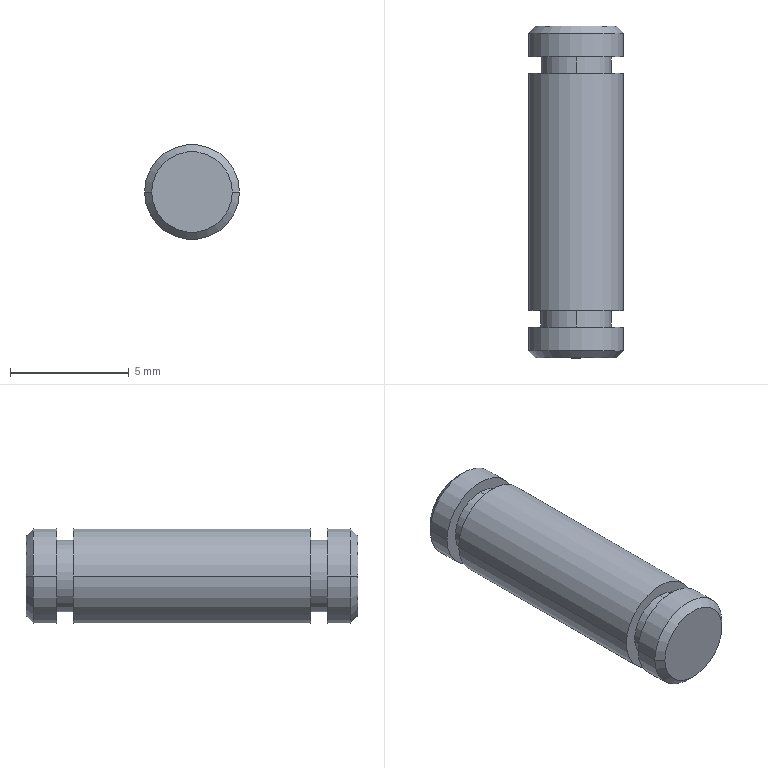Part | NX | 1 solid | 20 faces | box 4 x 14 x 4 mm | volume 167.158 mm3 | cylinder 10 | plane 6 | cone 4 | commonest cylinder face diameters 4 x6 3 x4
STEP:
#1=CARTESIAN_POINT('',(-42.,151.3,-84.4));
#2=VERTEX_POINT('',#1);
#3=CARTESIAN_POINT('',(-46.,151.3,-84.4));
#4=VERTEX_POINT('',#3);
#5=CARTESIAN_POINT('',(-44.,151.3,-84.4));
#6=DIRECTION('',(0.,1.,0.));
#7=DIRECTION('',(-1.,0.,0.));
#8=AXIS2_PLACEMENT_3D('',#5,#6,#7);
#9=CIRCLE('',#8,2.);
#10=EDGE_CURVE('',#2,#4,#9,.T.);
#11=ORIENTED_EDGE('',*,*,#10,.T.);
#12=CARTESIAN_POINT('',(-46.,152.3,-84.4));
#13=VERTEX_POINT('',#12);
#14=CARTESIAN_POINT('',(-46.,165.,-84.4));
#15=DIRECTION('',(0.,1.,0.));
#16=VECTOR('',#15,1000.);
#17=LINE('',#14,#16);
#18=EDGE_CURVE('',#4,#13,#17,.T.);
#19=ORIENTED_EDGE('',*,*,#18,.T.);
#20=CARTESIAN_POINT('',(-42.,152.3,-84.4));
#21=VERTEX_POINT('',#20);
#22=CARTESIAN_POINT('',(-44.,152.3,-84.4));
#23=DIRECTION('',(0.,1.,0.));
#24=DIRECTION('',(-1.,0.,0.));
#25=AXIS2_PLACEMENT_3D('',#22,#23,#24);
#26=CIRCLE('',#25,2.);
#27=EDGE_CURVE('',#21,#13,#26,.T.);
#28=ORIENTED_EDGE('',*,*,#27,.F.);
#29=CARTESIAN_POINT('',(-42.,165.,-84.4));
#30=DIRECTION('',(0.,1.,0.));
#31=VECTOR('',#30,1000.);
#32=LINE('',#29,#31);
#33=EDGE_CURVE('',#2,#21,#32,.T.);
#34=ORIENTED_EDGE('',*,*,#33,.F.);
#35=EDGE_LOOP('',(#11,#19,#28,#34));
#36=FACE_BOUND('',#35,.T.);
#37=CARTESIAN_POINT('',(-44.,165.,-84.4));
#38=DIRECTION('',(0.,1.,0.));
#39=DIRECTION('',(-1.,0.,0.));
#40=AXIS2_PLACEMENT_3D('',#37,#38,#39);
#41=CYLINDRICAL_SURFACE('',#40,2.);
#42=ADVANCED_FACE('',(#36),#41,.T.);
#43=CARTESIAN_POINT('',(-42.,163.7,-84.4));
#44=VERTEX_POINT('',#43);
#45=CARTESIAN_POINT('',(-46.,163.7,-84.4));
#46=VERTEX_POINT('',#45);
#47=CARTESIAN_POINT('',(-44.,163.7,-84.4));
#48=DIRECTION('',(0.,1.,0.));
#49=DIRECTION('',(-1.,0.,0.));
#50=AXIS2_PLACEMENT_3D('',#47,#48,#49);
#51=CIRCLE('',#50,2.);
#52=EDGE_CURVE('',#44,#46,#51,.T.);
#53=ORIENTED_EDGE('',*,*,#52,.T.);
#54=CARTESIAN_POINT('',(-46.,164.7,-84.4));
#55=VERTEX_POINT('',#54);
#56=CARTESIAN_POINT('',(-46.,165.,-84.4));
#57=DIRECTION('',(0.,1.,0.));
#58=VECTOR('',#57,1000.);
#59=LINE('',#56,#58);
#60=EDGE_CURVE('',#55,#46,#59,.F.);
#61=ORIENTED_EDGE('',*,*,#60,.F.);
#62=CARTESIAN_POINT('',(-42.,164.7,-84.4));
#63=VERTEX_POINT('',#62);
#64=CARTESIAN_POINT('',(-44.,164.7,-84.4));
#65=DIRECTION('',(0.,1.,0.));
#66=DIRECTION('',(-1.,0.,0.));
#67=AXIS2_PLACEMENT_3D('',#64,#65,#66);
#68=CIRCLE('',#67,2.);
#69=EDGE_CURVE('',#63,#55,#68,.T.);
#70=ORIENTED_EDGE('',*,*,#69,.F.);
#71=CARTESIAN_POINT('',(-42.,165.,-84.4));
#72=DIRECTION('',(0.,1.,0.));
#73=VECTOR('',#72,1000.);
#74=LINE('',#71,#73);
#75=EDGE_CURVE('',#63,#44,#74,.F.);
#76=ORIENTED_EDGE('',*,*,#75,.T.);
#77=EDGE_LOOP('',(#53,#61,#70,#76));
#78=FACE_BOUND('',#77,.T.);
#79=CARTESIAN_POINT('',(-44.,165.,-84.4));
#80=DIRECTION('',(0.,1.,0.));
#81=DIRECTION('',(-1.,0.,0.));
#82=AXIS2_PLACEMENT_3D('',#79,#80,#81);
#83=CYLINDRICAL_SURFACE('',#82,2.);
#84=ADVANCED_FACE('',(#78),#83,.T.);
#85=CARTESIAN_POINT('',(-42.,153.,-84.4));
#86=VERTEX_POINT('',#85);
#87=CARTESIAN_POINT('',(-46.,153.,-84.4));
#88=VERTEX_POINT('',#87);
#89=CARTESIAN_POINT('',(-44.,153.,-84.4));
#90=DIRECTION('',(0.,1.,0.));
#91=DIRECTION('',(-1.,0.,0.));
#92=AXIS2_PLACEMENT_3D('',#89,#90,#91);
#93=CIRCLE('',#92,2.);
#94=EDGE_CURVE('',#86,#88,#93,.T.);
#95=ORIENTED_EDGE('',*,*,#94,.T.);
#96=CARTESIAN_POINT('',(-46.,163.,-84.4));
#97=VERTEX_POINT('',#96);
#98=CARTESIAN_POINT('',(-46.,165.,-84.4));
#99=DIRECTION('',(0.,1.,0.));
#100=VECTOR('',#99,1000.);
#101=LINE('',#98,#100);
#102=EDGE_CURVE('',#97,#88,#101,.F.);
#103=ORIENTED_EDGE('',*,*,#102,.F.);
#104=CARTESIAN_POINT('',(-42.,163.,-84.4));
#105=VERTEX_POINT('',#104);
#106=CARTESIAN_POINT('',(-44.,163.,-84.4));
#107=DIRECTION('',(0.,1.,0.));
#108=DIRECTION('',(-1.,0.,0.));
#109=AXIS2_PLACEMENT_3D('',#106,#107,#108);
#110=CIRCLE('',#109,2.);
#111=EDGE_CURVE('',#105,#97,#110,.T.);
#112=ORIENTED_EDGE('',*,*,#111,.F.);
#113=CARTESIAN_POINT('',(-42.,165.,-84.4));
#114=DIRECTION('',(0.,1.,0.));
#115=VECTOR('',#114,1000.);
#116=LINE('',#113,#115);
#117=EDGE_CURVE('',#105,#86,#116,.F.);
#118=ORIENTED_EDGE('',*,*,#117,.T.);
#119=EDGE_LOOP('',(#95,#103,#112,#118));
#120=FACE_BOUND('',#119,.T.);
#121=CARTESIAN_POINT('',(-44.,165.,-84.4));
#122=DIRECTION('',(0.,1.,0.));
#123=DIRECTION('',(-1.,0.,0.));
#124=AXIS2_PLACEMENT_3D('',#121,#122,#123);
#125=CYLINDRICAL_SURFACE('',#124,2.);
#126=ADVANCED_FACE('',(#120),#125,.T.);
#127=ORIENTED_EDGE('',*,*,#52,.F.);
#128=CARTESIAN_POINT('',(-44.,163.7,-84.4));
#129=DIRECTION('',(0.,1.,0.));
#130=DIRECTION('',(-1.,0.,0.));
#131=AXIS2_PLACEMENT_3D('',#128,#129,#130);
#132=CIRCLE('',#131,2.);
#133=EDGE_CURVE('',#46,#44,#132,.T.);
#134=ORIENTED_EDGE('',*,*,#133,.F.);
#135=EDGE_LOOP('',(#127,#134));
#136=FACE_BOUND('',#135,.T.);
#137=CARTESIAN_POINT('',(-44.,163.7,-82.9));
#138=VERTEX_POINT('',#137);
#139=CARTESIAN_POINT('',(-44.,163.7,-85.9));
#140=VERTEX_POINT('',#139);
#141=CARTESIAN_POINT('',(-44.,163.7,-84.4));
#142=DIRECTION('',(0.,1.,0.));
#143=DIRECTION('',(1.,0.,0.));
#144=AXIS2_PLACEMENT_3D('',#141,#142,#143);
#145=CIRCLE('',#144,1.5);
#146=EDGE_CURVE('',#138,#140,#145,.T.);
#147=ORIENTED_EDGE('',*,*,#146,.T.);
#148=CARTESIAN_POINT('',(-44.,163.7,-84.4));
#149=DIRECTION('',(0.,1.,0.));
#150=DIRECTION('',(1.,0.,0.));
#151=AXIS2_PLACEMENT_3D('',#148,#149,#150);
#152=CIRCLE('',#151,1.5);
#153=EDGE_CURVE('',#140,#138,#152,.T.);
#154=ORIENTED_EDGE('',*,*,#153,.T.);
#155=EDGE_LOOP('',(#147,#154));
#156=FACE_BOUND('',#155,.T.);
#157=CARTESIAN_POINT('',(-41.314,163.7,-84.4));
#158=DIRECTION('',(0.,1.,0.));
#159=DIRECTION('',(0.,0.,-1.));
#160=AXIS2_PLACEMENT_3D('',#157,#158,#159);
#161=PLANE('',#160);
#162=ADVANCED_FACE('',(#136,#156),#161,.F.);
#163=ORIENTED_EDGE('',*,*,#146,.F.);
#164=CARTESIAN_POINT('',(-44.,163.,-82.9));
#165=VERTEX_POINT('',#164);
#166=CARTESIAN_POINT('',(-44.,163.35,-82.9));
#167=DIRECTION('',(0.,1.,0.));
#168=VECTOR('',#167,1000.);
#169=LINE('',#166,#168);
#170=EDGE_CURVE('',#165,#138,#169,.T.);
#171=ORIENTED_EDGE('',*,*,#170,.F.);
#172=CARTESIAN_POINT('',(-44.,163.,-85.9));
#173=VERTEX_POINT('',#172);
#174=CARTESIAN_POINT('',(-44.,163.,-84.4));
#175=DIRECTION('',(0.,1.,0.));
#176=DIRECTION('',(1.,0.,0.));
#177=AXIS2_PLACEMENT_3D('',#174,#175,#176);
#178=CIRCLE('',#177,1.5);
#179=EDGE_CURVE('',#165,#173,#178,.T.);
#180=ORIENTED_EDGE('',*,*,#179,.T.);
#181=CARTESIAN_POINT('',(-44.,163.35,-85.9));
#182=DIRECTION('',(0.,1.,0.));
#183=VECTOR('',#182,1000.);
#184=LINE('',#181,#183);
#185=EDGE_CURVE('',#173,#140,#184,.T.);
#186=ORIENTED_EDGE('',*,*,#185,.T.);
#187=EDGE_LOOP('',(#163,#171,#180,#186));
#188=FACE_BOUND('',#187,.T.);
#189=CARTESIAN_POINT('',(-44.,163.35,-84.4));
#190=DIRECTION('',(0.,1.,0.));
#191=DIRECTION('',(0.,0.,1.));
#192=AXIS2_PLACEMENT_3D('',#189,#190,#191);
#193=CYLINDRICAL_SURFACE('',#192,1.5);
#194=ADVANCED_FACE('',(#188),#193,.T.);
#195=CARTESIAN_POINT('',(-44.,163.,-84.4));
#196=DIRECTION('',(0.,1.,0.));
#197=DIRECTION('',(-1.,0.,0.));
#198=AXIS2_PLACEMENT_3D('',#195,#196,#197);
#199=CIRCLE('',#198,2.);
#200=EDGE_CURVE('',#97,#105,#199,.T.);
#201=ORIENTED_EDGE('',*,*,#200,.T.);
#202=ORIENTED_EDGE('',*,*,#111,.T.);
#203=EDGE_LOOP('',(#201,#202));
#204=FACE_BOUND('',#203,.T.);
#205=ORIENTED_EDGE('',*,*,#179,.F.);
#206=CARTESIAN_POINT('',(-44.,163.,-84.4));
#207=DIRECTION('',(0.,1.,0.));
#208=DIRECTION('',(1.,0.,0.));
#209=AXIS2_PLACEMENT_3D('',#206,#207,#208);
#210=CIRCLE('',#209,1.5);
#211=EDGE_CURVE('',#173,#165,#210,.T.);
#212=ORIENTED_EDGE('',*,*,#211,.F.);
#213=EDGE_LOOP('',(#205,#212));
#214=FACE_BOUND('',#213,.T.);
#215=CARTESIAN_POINT('',(-42.25,163.,-84.4));
#216=DIRECTION('',(0.,-1.,0.));
#217=DIRECTION('',(-1.,0.,0.));
#218=AXIS2_PLACEMENT_3D('',#215,#216,#217);
#219=PLANE('',#218);
#220=ADVANCED_FACE('',(#204,#214),#219,.F.);
#221=ORIENTED_EDGE('',*,*,#94,.F.);
#222=CARTESIAN_POINT('',(-44.,153.,-84.4));
#223=DIRECTION('',(0.,1.,0.));
#224=DIRECTION('',(-1.,0.,0.));
#225=AXIS2_PLACEMENT_3D('',#222,#223,#224);
#226=CIRCLE('',#225,2.);
#227=EDGE_CURVE('',#88,#86,#226,.T.);
#228=ORIENTED_EDGE('',*,*,#227,.F.);
#229=EDGE_LOOP('',(#221,#228));
#230=FACE_BOUND('',#229,.T.);
#231=CARTESIAN_POINT('',(-44.,153.,-85.9));
#232=VERTEX_POINT('',#231);
#233=CARTESIAN_POINT('',(-44.,153.,-82.9));
#234=VERTEX_POINT('',#233);
#235=CARTESIAN_POINT('',(-44.,153.,-84.4));
#236=DIRECTION('',(0.,1.,0.));
#237=DIRECTION('',(0.,0.,1.));
#238=AXIS2_PLACEMENT_3D('',#235,#236,#237);
#239=CIRCLE('',#238,1.5);
#240=EDGE_CURVE('',#232,#234,#239,.T.);
#241=ORIENTED_EDGE('',*,*,#240,.T.);
#242=CARTESIAN_POINT('',(-44.,153.,-84.4));
#243=DIRECTION('',(0.,1.,0.));
#244=DIRECTION('',(0.,0.,1.));
#245=AXIS2_PLACEMENT_3D('',#242,#243,#244);
#246=CIRCLE('',#245,1.5);
#247=EDGE_CURVE('',#234,#232,#246,.T.);
#248=ORIENTED_EDGE('',*,*,#247,.T.);
#249=EDGE_LOOP('',(#241,#248));
#250=FACE_BOUND('',#249,.T.);
#251=CARTESIAN_POINT('',(-42.25,153.,-84.4));
#252=DIRECTION('',(0.,1.,0.));
#253=DIRECTION('',(0.,0.,-1.));
#254=AXIS2_PLACEMENT_3D('',#251,#252,#253);
#255=PLANE('',#254);
#256=ADVANCED_FACE('',(#230,#250),#255,.F.);
#257=ORIENTED_EDGE('',*,*,#240,.F.);
#258=CARTESIAN_POINT('',(-44.,152.3,-85.9));
#259=VERTEX_POINT('',#258);
#260=CARTESIAN_POINT('',(-44.,154.65,-85.9));
#261=DIRECTION('',(0.,1.,0.));
#262=VECTOR('',#261,1000.);
#263=LINE('',#260,#262);
#264=EDGE_CURVE('',#259,#232,#263,.T.);
#265=ORIENTED_EDGE('',*,*,#264,.F.);
#266=CARTESIAN_POINT('',(-44.,152.3,-82.9));
#267=VERTEX_POINT('',#266);
#268=CARTESIAN_POINT('',(-44.,152.3,-84.4));
#269=DIRECTION('',(0.,1.,0.));
#270=DIRECTION('',(0.,0.,1.));
#271=AXIS2_PLACEMENT_3D('',#268,#269,#270);
#272=CIRCLE('',#271,1.5);
#273=EDGE_CURVE('',#259,#267,#272,.T.);
#274=ORIENTED_EDGE('',*,*,#273,.T.);
#275=CARTESIAN_POINT('',(-44.,154.65,-82.9));
#276=DIRECTION('',(0.,1.,0.));
#277=VECTOR('',#276,1000.);
#278=LINE('',#275,#277);
#279=EDGE_CURVE('',#267,#234,#278,.T.);
#280=ORIENTED_EDGE('',*,*,#279,.T.);
#281=EDGE_LOOP('',(#257,#265,#274,#280));
#282=FACE_BOUND('',#281,.T.);
#283=CARTESIAN_POINT('',(-44.,154.65,-84.4));
#284=DIRECTION('',(0.,1.,0.));
#285=DIRECTION('',(0.,0.,1.));
#286=AXIS2_PLACEMENT_3D('',#283,#284,#285);
#287=CYLINDRICAL_SURFACE('',#286,1.5);
#288=ADVANCED_FACE('',(#282),#287,.T.);
#289=ORIENTED_EDGE('',*,*,#27,.T.);
#290=CARTESIAN_POINT('',(-44.,152.3,-84.4));
#291=DIRECTION('',(0.,1.,0.));
#292=DIRECTION('',(-1.,0.,0.));
#293=AXIS2_PLACEMENT_3D('',#290,#291,#292);
#294=CIRCLE('',#293,2.);
#295=EDGE_CURVE('',#13,#21,#294,.T.);
#296=ORIENTED_EDGE('',*,*,#295,.T.);
#297=EDGE_LOOP('',(#289,#296));
#298=FACE_BOUND('',#297,.T.);
#299=ORIENTED_EDGE('',*,*,#273,.F.);
#300=CARTESIAN_POINT('',(-44.,152.3,-84.4));
#301=DIRECTION('',(0.,1.,0.));
#302=DIRECTION('',(0.,0.,1.));
#303=AXIS2_PLACEMENT_3D('',#300,#301,#302);
#304=CIRCLE('',#303,1.5);
#305=EDGE_CURVE('',#267,#259,#304,.T.);
#306=ORIENTED_EDGE('',*,*,#305,.F.);
#307=EDGE_LOOP('',(#299,#306));
#308=FACE_BOUND('',#307,.T.);
#309=CARTESIAN_POINT('',(-41.396,152.3,-84.4));
#310=DIRECTION('',(0.,1.,0.));
#311=DIRECTION('',(0.,0.,-1.));
#312=AXIS2_PLACEMENT_3D('',#309,#310,#311);
#313=PLANE('',#312);
#314=ADVANCED_FACE('',(#298,#308),#313,.T.);
#315=ORIENTED_EDGE('',*,*,#279,.F.);
#316=ORIENTED_EDGE('',*,*,#305,.T.);
#317=ORIENTED_EDGE('',*,*,#264,.T.);
#318=ORIENTED_EDGE('',*,*,#247,.F.);
#319=EDGE_LOOP('',(#315,#316,#317,#318));
#320=FACE_BOUND('',#319,.T.);
#321=CARTESIAN_POINT('',(-44.,154.65,-84.4));
#322=DIRECTION('',(0.,1.,0.));
#323=DIRECTION('',(0.,0.,1.));
#324=AXIS2_PLACEMENT_3D('',#321,#322,#323);
#325=CYLINDRICAL_SURFACE('',#324,1.5);
#326=ADVANCED_FACE('',(#320),#325,.T.);
#327=ORIENTED_EDGE('',*,*,#60,.T.);
#328=ORIENTED_EDGE('',*,*,#133,.T.);
#329=ORIENTED_EDGE('',*,*,#75,.F.);
#330=CARTESIAN_POINT('',(-44.,164.7,-84.4));
#331=DIRECTION('',(0.,1.,0.));
#332=DIRECTION('',(-1.,0.,0.));
#333=AXIS2_PLACEMENT_3D('',#330,#331,#332);
#334=CIRCLE('',#333,2.);
#335=EDGE_CURVE('',#55,#63,#334,.T.);
#336=ORIENTED_EDGE('',*,*,#335,.F.);
#337=EDGE_LOOP('',(#327,#328,#329,#336));
#338=FACE_BOUND('',#337,.T.);
#339=CARTESIAN_POINT('',(-44.,165.,-84.4));
#340=DIRECTION('',(0.,1.,0.));
#341=DIRECTION('',(-1.,0.,0.));
#342=AXIS2_PLACEMENT_3D('',#339,#340,#341);
#343=CYLINDRICAL_SURFACE('',#342,2.);
#344=ADVANCED_FACE('',(#338),#343,.T.);
#345=ORIENTED_EDGE('',*,*,#170,.T.);
#346=ORIENTED_EDGE('',*,*,#153,.F.);
#347=ORIENTED_EDGE('',*,*,#185,.F.);
#348=ORIENTED_EDGE('',*,*,#211,.T.);
#349=EDGE_LOOP('',(#345,#346,#347,#348));
#350=FACE_BOUND('',#349,.T.);
#351=CARTESIAN_POINT('',(-44.,163.35,-84.4));
#352=DIRECTION('',(0.,1.,0.));
#353=DIRECTION('',(0.,0.,1.));
#354=AXIS2_PLACEMENT_3D('',#351,#352,#353);
#355=CYLINDRICAL_SURFACE('',#354,1.5);
#356=ADVANCED_FACE('',(#350),#355,.T.);
#357=ORIENTED_EDGE('',*,*,#33,.T.);
#358=ORIENTED_EDGE('',*,*,#295,.F.);
#359=ORIENTED_EDGE('',*,*,#18,.F.);
#360=CARTESIAN_POINT('',(-44.,151.3,-84.4));
#361=DIRECTION('',(0.,1.,0.));
#362=DIRECTION('',(-1.,0.,0.));
#363=AXIS2_PLACEMENT_3D('',#360,#361,#362);
#364=CIRCLE('',#363,2.);
#365=EDGE_CURVE('',#4,#2,#364,.T.);
#366=ORIENTED_EDGE('',*,*,#365,.T.);
#367=EDGE_LOOP('',(#357,#358,#359,#366));
#368=FACE_BOUND('',#367,.T.);
#369=CARTESIAN_POINT('',(-44.,165.,-84.4));
#370=DIRECTION('',(0.,1.,0.));
#371=DIRECTION('',(-1.,0.,0.));
#372=AXIS2_PLACEMENT_3D('',#369,#370,#371);
#373=CYLINDRICAL_SURFACE('',#372,2.);
#374=ADVANCED_FACE('',(#368),#373,.T.);
#375=ORIENTED_EDGE('',*,*,#200,.F.);
#376=ORIENTED_EDGE('',*,*,#102,.T.);
#377=ORIENTED_EDGE('',*,*,#227,.T.);
#378=ORIENTED_EDGE('',*,*,#117,.F.);
#379=EDGE_LOOP('',(#375,#376,#377,#378));
#380=FACE_BOUND('',#379,.T.);
#381=CARTESIAN_POINT('',(-44.,165.,-84.4));
#382=DIRECTION('',(0.,1.,0.));
#383=DIRECTION('',(-1.,0.,0.));
#384=AXIS2_PLACEMENT_3D('',#381,#382,#383);
#385=CYLINDRICAL_SURFACE('',#384,2.);
#386=ADVANCED_FACE('',(#380),#385,.T.);
#387=CARTESIAN_POINT('',(-42.3,151.,-84.4));
#388=VERTEX_POINT('',#387);
#389=CARTESIAN_POINT('',(-45.7,151.,-84.4));
#390=VERTEX_POINT('',#389);
#391=CARTESIAN_POINT('',(-44.,151.,-84.4));
#392=DIRECTION('',(0.,1.,0.));
#393=DIRECTION('',(-1.,0.,0.));
#394=AXIS2_PLACEMENT_3D('',#391,#392,#393);
#395=CIRCLE('',#394,1.7);
#396=EDGE_CURVE('',#388,#390,#395,.T.);
#397=ORIENTED_EDGE('',*,*,#396,.F.);
#398=CARTESIAN_POINT('',(-44.,151.,-84.4));
#399=DIRECTION('',(0.,1.,0.));
#400=DIRECTION('',(-1.,0.,0.));
#401=AXIS2_PLACEMENT_3D('',#398,#399,#400);
#402=CIRCLE('',#401,1.7);
#403=EDGE_CURVE('',#390,#388,#402,.T.);
#404=ORIENTED_EDGE('',*,*,#403,.F.);
#405=EDGE_LOOP('',(#397,#404));
#406=FACE_BOUND('',#405,.T.);
#407=CARTESIAN_POINT('',(-42.256,151.,-78.065));
#408=DIRECTION('',(0.,1.,0.));
#409=DIRECTION('',(0.,0.,-1.));
#410=AXIS2_PLACEMENT_3D('',#407,#408,#409);
#411=PLANE('',#410);
#412=ADVANCED_FACE('',(#406),#411,.F.);
#413=ORIENTED_EDGE('',*,*,#396,.T.);
#414=CARTESIAN_POINT('',(-45.7,151.,-84.4));
#415=DIRECTION('',(-0.7071,0.7071,0.));
#416=VECTOR('',#415,1000.);
#417=LINE('',#414,#416);
#418=EDGE_CURVE('',#4,#390,#417,.F.);
#419=ORIENTED_EDGE('',*,*,#418,.F.);
#420=ORIENTED_EDGE('',*,*,#10,.F.);
#421=CARTESIAN_POINT('',(-42.3,151.,-84.4));
#422=DIRECTION('',(0.7071,0.7071,0.));
#423=VECTOR('',#422,1000.);
#424=LINE('',#421,#423);
#425=EDGE_CURVE('',#2,#388,#424,.F.);
#426=ORIENTED_EDGE('',*,*,#425,.T.);
#427=EDGE_LOOP('',(#413,#419,#420,#426));
#428=FACE_BOUND('',#427,.T.);
#429=CARTESIAN_POINT('',(-44.,151.,-84.4));
#430=DIRECTION('',(0.,1.,0.));
#431=DIRECTION('',(-1.,0.,0.));
#432=AXIS2_PLACEMENT_3D('',#429,#430,#431);
#433=CONICAL_SURFACE('',#432,1.7,0.7854);
#434=ADVANCED_FACE('',(#428),#433,.T.);
#435=ORIENTED_EDGE('',*,*,#418,.T.);
#436=ORIENTED_EDGE('',*,*,#403,.T.);
#437=ORIENTED_EDGE('',*,*,#425,.F.);
#438=ORIENTED_EDGE('',*,*,#365,.F.);
#439=EDGE_LOOP('',(#435,#436,#437,#438));
#440=FACE_BOUND('',#439,.T.);
#441=CARTESIAN_POINT('',(-44.,151.,-84.4));
#442=DIRECTION('',(0.,1.,0.));
#443=DIRECTION('',(-1.,0.,0.));
#444=AXIS2_PLACEMENT_3D('',#441,#442,#443);
#445=CONICAL_SURFACE('',#444,1.7,0.7854);
#446=ADVANCED_FACE('',(#440),#445,.T.);
#447=CARTESIAN_POINT('',(-42.3,165.,-84.4));
#448=VERTEX_POINT('',#447);
#449=CARTESIAN_POINT('',(-45.7,165.,-84.4));
#450=VERTEX_POINT('',#449);
#451=CARTESIAN_POINT('',(-44.,165.,-84.4));
#452=DIRECTION('',(0.,1.,0.));
#453=DIRECTION('',(-1.,0.,0.));
#454=AXIS2_PLACEMENT_3D('',#451,#452,#453);
#455=CIRCLE('',#454,1.7);
#456=EDGE_CURVE('',#448,#450,#455,.T.);
#457=ORIENTED_EDGE('',*,*,#456,.T.);
#458=CARTESIAN_POINT('',(-44.,165.,-84.4));
#459=DIRECTION('',(0.,1.,0.));
#460=DIRECTION('',(-1.,0.,0.));
#461=AXIS2_PLACEMENT_3D('',#458,#459,#460);
#462=CIRCLE('',#461,1.7);
#463=EDGE_CURVE('',#450,#448,#462,.T.);
#464=ORIENTED_EDGE('',*,*,#463,.T.);
#465=EDGE_LOOP('',(#457,#464));
#466=FACE_BOUND('',#465,.T.);
#467=CARTESIAN_POINT('',(-42.256,165.,-78.065));
#468=DIRECTION('',(0.,1.,0.));
#469=DIRECTION('',(0.,0.,-1.));
#470=AXIS2_PLACEMENT_3D('',#467,#468,#469);
#471=PLANE('',#470);
#472=ADVANCED_FACE('',(#466),#471,.T.);
#473=ORIENTED_EDGE('',*,*,#456,.F.);
#474=CARTESIAN_POINT('',(-42.3,165.,-84.4));
#475=DIRECTION('',(0.7071,-0.7071,0.));
#476=VECTOR('',#475,1000.);
#477=LINE('',#474,#476);
#478=EDGE_CURVE('',#448,#63,#477,.T.);
#479=ORIENTED_EDGE('',*,*,#478,.T.);
#480=ORIENTED_EDGE('',*,*,#69,.T.);
#481=CARTESIAN_POINT('',(-45.7,165.,-84.4));
#482=DIRECTION('',(-0.7071,-0.7071,0.));
#483=VECTOR('',#482,1000.);
#484=LINE('',#481,#483);
#485=EDGE_CURVE('',#450,#55,#484,.T.);
#486=ORIENTED_EDGE('',*,*,#485,.F.);
#487=EDGE_LOOP('',(#473,#479,#480,#486));
#488=FACE_BOUND('',#487,.T.);
#489=CARTESIAN_POINT('',(-44.,165.,-84.4));
#490=DIRECTION('',(0.,-1.,0.));
#491=DIRECTION('',(1.,0.,0.));
#492=AXIS2_PLACEMENT_3D('',#489,#490,#491);
#493=CONICAL_SURFACE('',#492,1.7,0.7854);
#494=ADVANCED_FACE('',(#488),#493,.T.);
#495=ORIENTED_EDGE('',*,*,#478,.F.);
#496=ORIENTED_EDGE('',*,*,#463,.F.);
#497=ORIENTED_EDGE('',*,*,#485,.T.);
#498=ORIENTED_EDGE('',*,*,#335,.T.);
#499=EDGE_LOOP('',(#495,#496,#497,#498));
#500=FACE_BOUND('',#499,.T.);
#501=CARTESIAN_POINT('',(-44.,165.,-84.4));
#502=DIRECTION('',(0.,-1.,0.));
#503=DIRECTION('',(1.,0.,0.));
#504=AXIS2_PLACEMENT_3D('',#501,#502,#503);
#505=CONICAL_SURFACE('',#504,1.7,0.7854);
#506=ADVANCED_FACE('',(#500),#505,.T.);
#507=CLOSED_SHELL('',(#42,#84,#126,#162,#194,#220,#256,#288,#314,#326,#344,#356,#374,#386,#412,#434,#446,#472,#494,#506));
#508=MANIFOLD_SOLID_BREP('',#507);
#509=(LENGTH_UNIT()NAMED_UNIT(*)SI_UNIT(.MILLI.,.METRE.));
#510=UNCERTAINTY_MEASURE_WITH_UNIT(LENGTH_MEASURE(0.00001),#509,'','');
#511=(NAMED_UNIT(*)PLANE_ANGLE_UNIT()SI_UNIT($,.RADIAN.));
#512=(NAMED_UNIT(*)SI_UNIT($,.STERADIAN.)SOLID_ANGLE_UNIT());
#513=(GEOMETRIC_REPRESENTATION_CONTEXT(3)GLOBAL_UNCERTAINTY_ASSIGNED_CONTEXT((#510))GLOBAL_UNIT_ASSIGNED_CONTEXT((#509,#511,#512))REPRESENTATION_CONTEXT('',''));
#514=ADVANCED_BREP_SHAPE_REPRESENTATION('',(#508),#513);